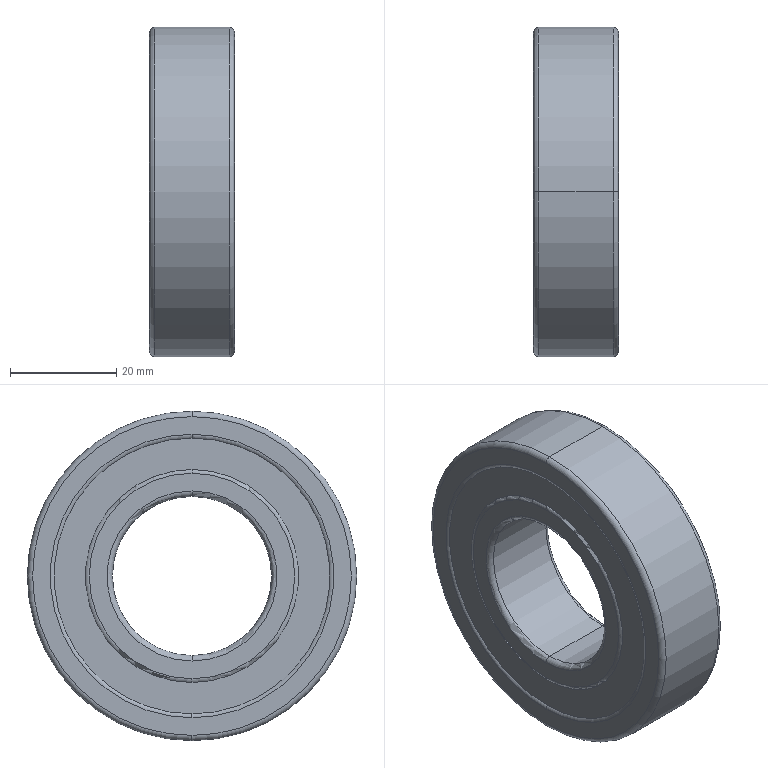Part | SolidWorks | features Revolution 5, CirPattern 2, RefAxis 1, RevCut 1 | 16 solids | 184 faces | box 16 x 62 x 62 mm | volume 27684 mm3 | cylinder 66 | sphere 60 | plane 34 | torus 24 | commonest cylinder face diameters 44.4 x27 47.6 x27 40.667 x4 51.333 x4 30 x2 62 x2